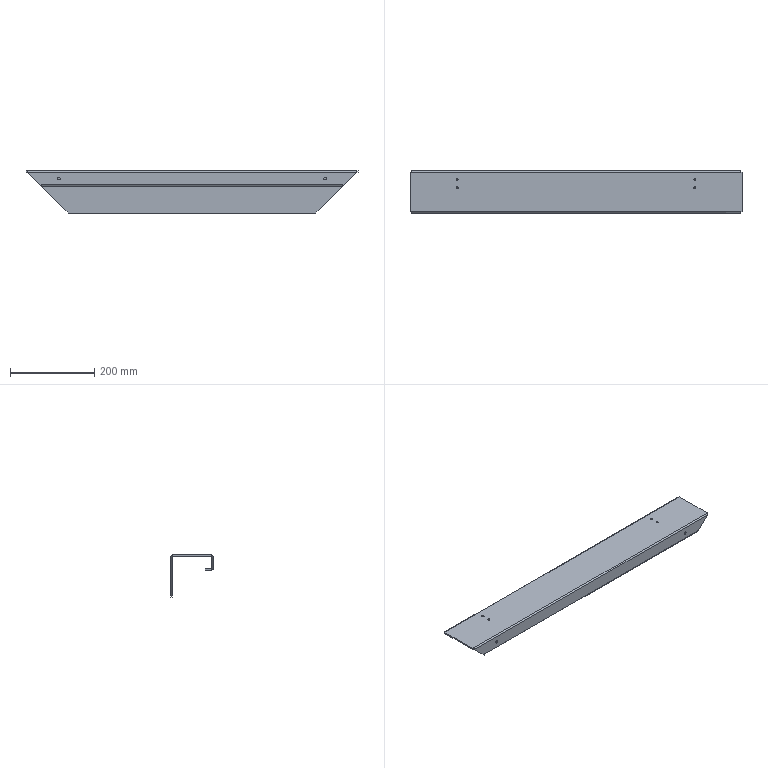Part | STEP file | HESS-408-70-15W-W-11-bottom frame 1 | 1 solid | 56 faces | box 790 x 100 x 100 mm | volume 538062 mm3 | plane 30 | cylinder 22 | spline 4 | commonest cylinder face diameters 5 x8 6.8 x8 0.2 x3 6.2 x3